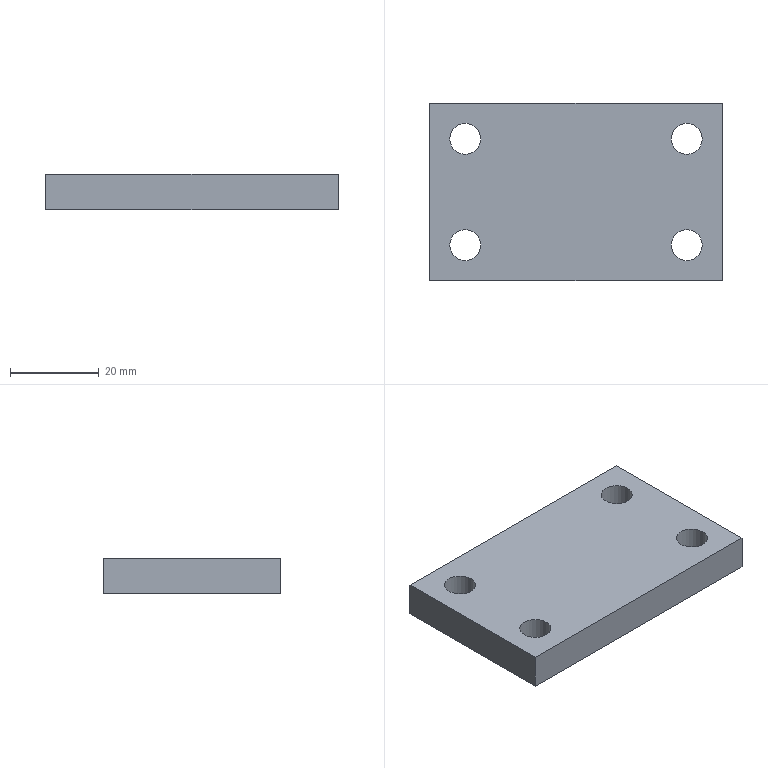Part | STEP file | Tube feed_id1018_x_t | 1 solid | 10 faces | box 66 x 40 x 8 mm | volume 19888 mm3 | plane 6 | cylinder 4 | commonest cylinder face diameters 7 x4
STEP:
#1=CARTESIAN_POINT('',(0.,0.,0.));
#2=DIRECTION('',(0.,0.,1.));
#3=DIRECTION('',(1.,0.,0.));
#4=AXIS2_PLACEMENT_3D('',#1,#2,#3);
#5=CARTESIAN_POINT('',(-297.,53.975,-133.5));
#6=VERTEX_POINT('',#5);
#7=CARTESIAN_POINT('',(-293.5,53.975,-133.5));
#8=DIRECTION('',(0.,0.,-1.));
#9=DIRECTION('',(-1.,0.,0.));
#10=AXIS2_PLACEMENT_3D('',#7,#8,#9);
#11=CIRCLE('',#10,3.5);
#12=CARTESIAN_POINT('',(-235.5,21.975,-133.5));
#13=DIRECTION('',(0.,0.,1.));
#14=DIRECTION('',(-1.,0.,0.));
#15=AXIS2_PLACEMENT_3D('',#12,#13,#14);
#16=PLANE('',#15);
#17=CARTESIAN_POINT('',(61.5,-32.));
#18=CARTESIAN_POINT('',(61.5,-38.062));
#19=CARTESIAN_POINT('',(56.25,-35.031));
#20=CARTESIAN_POINT('',(51.,-32.));
#21=CARTESIAN_POINT('',(56.25,-28.969));
#22=CARTESIAN_POINT('',(61.5,-25.938));
#23=CARTESIAN_POINT('',(61.5,-32.));
#24=(BOUNDED_CURVE()B_SPLINE_CURVE(2,(#17,#18,#19,#20,#21,#22,#23),.UNSPECIFIED.,.T.,.F.)B_SPLINE_CURVE_WITH_KNOTS((1,2,2,2,2,1),(-2.094,0.,2.094,4.189,6.283,8.378),.UNSPECIFIED.)CURVE()GEOMETRIC_REPRESENTATION_ITEM()RATIONAL_B_SPLINE_CURVE((1.,0.5,1.,0.5,1.,0.5,1.))REPRESENTATION_ITEM(''));
#25=(GEOMETRIC_REPRESENTATION_CONTEXT(2)PARAMETRIC_REPRESENTATION_CONTEXT()REPRESENTATION_CONTEXT('',''));
#26=DEFINITIONAL_REPRESENTATION('',(#24),#25);
#27=PCURVE('',#16,#26);
#28=CARTESIAN_POINT('',(-293.5,53.975,-133.5));
#29=DIRECTION('',(0.,0.,-1.));
#30=DIRECTION('',(-1.,0.,0.));
#31=AXIS2_PLACEMENT_3D('',#28,#29,#30);
#32=CYLINDRICAL_SURFACE('',#31,3.5);
#33=CARTESIAN_POINT('',(0.,0.));
#34=DIRECTION('',(1.,0.));
#35=VECTOR('',#34,1.);
#36=LINE('',#33,#35);
#37=(GEOMETRIC_REPRESENTATION_CONTEXT(2)PARAMETRIC_REPRESENTATION_CONTEXT()REPRESENTATION_CONTEXT('',''));
#38=DEFINITIONAL_REPRESENTATION('',(#36),#37);
#39=PCURVE('',#32,#38);
#40=SURFACE_CURVE('',#11,(#27,#39),.PCURVE_S1.);
#41=EDGE_CURVE('',#6,#6,#40,.T.);
#42=ORIENTED_EDGE('',*,*,#41,.T.);
#43=EDGE_LOOP('',(#42));
#44=FACE_BOUND('',#43,.T.);
#45=CARTESIAN_POINT('',(-297.,29.975,-133.5));
#46=VERTEX_POINT('',#45);
#47=CARTESIAN_POINT('',(-293.5,29.975,-133.5));
#48=DIRECTION('',(0.,0.,-1.));
#49=DIRECTION('',(-1.,0.,0.));
#50=AXIS2_PLACEMENT_3D('',#47,#48,#49);
#51=CIRCLE('',#50,3.5);
#52=CARTESIAN_POINT('',(61.5,-8.));
#53=CARTESIAN_POINT('',(61.5,-14.062));
#54=CARTESIAN_POINT('',(56.25,-11.031));
#55=CARTESIAN_POINT('',(51.,-8.));
#56=CARTESIAN_POINT('',(56.25,-4.969));
#57=CARTESIAN_POINT('',(61.5,-1.938));
#58=CARTESIAN_POINT('',(61.5,-8.));
#59=(BOUNDED_CURVE()B_SPLINE_CURVE(2,(#52,#53,#54,#55,#56,#57,#58),.UNSPECIFIED.,.T.,.F.)B_SPLINE_CURVE_WITH_KNOTS((1,2,2,2,2,1),(-2.094,0.,2.094,4.189,6.283,8.378),.UNSPECIFIED.)CURVE()GEOMETRIC_REPRESENTATION_ITEM()RATIONAL_B_SPLINE_CURVE((1.,0.5,1.,0.5,1.,0.5,1.))REPRESENTATION_ITEM(''));
#60=(GEOMETRIC_REPRESENTATION_CONTEXT(2)PARAMETRIC_REPRESENTATION_CONTEXT()REPRESENTATION_CONTEXT('',''));
#61=DEFINITIONAL_REPRESENTATION('',(#59),#60);
#62=PCURVE('',#16,#61);
#63=CARTESIAN_POINT('',(-293.5,29.975,-133.5));
#64=DIRECTION('',(0.,0.,-1.));
#65=DIRECTION('',(-1.,0.,0.));
#66=AXIS2_PLACEMENT_3D('',#63,#64,#65);
#67=CYLINDRICAL_SURFACE('',#66,3.5);
#68=CARTESIAN_POINT('',(0.,0.));
#69=DIRECTION('',(1.,0.));
#70=VECTOR('',#69,1.);
#71=LINE('',#68,#70);
#72=(GEOMETRIC_REPRESENTATION_CONTEXT(2)PARAMETRIC_REPRESENTATION_CONTEXT()REPRESENTATION_CONTEXT('',''));
#73=DEFINITIONAL_REPRESENTATION('',(#71),#72);
#74=PCURVE('',#67,#73);
#75=SURFACE_CURVE('',#51,(#62,#74),.PCURVE_S1.);
#76=EDGE_CURVE('',#46,#46,#75,.T.);
#77=ORIENTED_EDGE('',*,*,#76,.T.);
#78=EDGE_LOOP('',(#77));
#79=FACE_BOUND('',#78,.T.);
#80=CARTESIAN_POINT('',(-247.,29.975,-133.5));
#81=VERTEX_POINT('',#80);
#82=CARTESIAN_POINT('',(-243.5,29.975,-133.5));
#83=DIRECTION('',(0.,0.,-1.));
#84=DIRECTION('',(-1.,0.,0.));
#85=AXIS2_PLACEMENT_3D('',#82,#83,#84);
#86=CIRCLE('',#85,3.5);
#87=CARTESIAN_POINT('',(11.5,-8.));
#88=CARTESIAN_POINT('',(11.5,-14.062));
#89=CARTESIAN_POINT('',(6.25,-11.031));
#90=CARTESIAN_POINT('',(1.,-8.));
#91=CARTESIAN_POINT('',(6.25,-4.969));
#92=CARTESIAN_POINT('',(11.5,-1.938));
#93=CARTESIAN_POINT('',(11.5,-8.));
#94=(BOUNDED_CURVE()B_SPLINE_CURVE(2,(#87,#88,#89,#90,#91,#92,#93),.UNSPECIFIED.,.T.,.F.)B_SPLINE_CURVE_WITH_KNOTS((1,2,2,2,2,1),(-2.094,0.,2.094,4.189,6.283,8.378),.UNSPECIFIED.)CURVE()GEOMETRIC_REPRESENTATION_ITEM()RATIONAL_B_SPLINE_CURVE((1.,0.5,1.,0.5,1.,0.5,1.))REPRESENTATION_ITEM(''));
#95=(GEOMETRIC_REPRESENTATION_CONTEXT(2)PARAMETRIC_REPRESENTATION_CONTEXT()REPRESENTATION_CONTEXT('',''));
#96=DEFINITIONAL_REPRESENTATION('',(#94),#95);
#97=PCURVE('',#16,#96);
#98=CARTESIAN_POINT('',(-243.5,29.975,-133.5));
#99=DIRECTION('',(0.,0.,-1.));
#100=DIRECTION('',(-1.,0.,0.));
#101=AXIS2_PLACEMENT_3D('',#98,#99,#100);
#102=CYLINDRICAL_SURFACE('',#101,3.5);
#103=CARTESIAN_POINT('',(0.,0.));
#104=DIRECTION('',(1.,0.));
#105=VECTOR('',#104,1.);
#106=LINE('',#103,#105);
#107=(GEOMETRIC_REPRESENTATION_CONTEXT(2)PARAMETRIC_REPRESENTATION_CONTEXT()REPRESENTATION_CONTEXT('',''));
#108=DEFINITIONAL_REPRESENTATION('',(#106),#107);
#109=PCURVE('',#102,#108);
#110=SURFACE_CURVE('',#86,(#97,#109),.PCURVE_S1.);
#111=EDGE_CURVE('',#81,#81,#110,.T.);
#112=ORIENTED_EDGE('',*,*,#111,.T.);
#113=EDGE_LOOP('',(#112));
#114=FACE_BOUND('',#113,.T.);
#115=CARTESIAN_POINT('',(-247.,53.975,-133.5));
#116=VERTEX_POINT('',#115);
#117=CARTESIAN_POINT('',(-243.5,53.975,-133.5));
#118=DIRECTION('',(0.,0.,-1.));
#119=DIRECTION('',(-1.,0.,0.));
#120=AXIS2_PLACEMENT_3D('',#117,#118,#119);
#121=CIRCLE('',#120,3.5);
#122=CARTESIAN_POINT('',(11.5,-32.));
#123=CARTESIAN_POINT('',(11.5,-38.062));
#124=CARTESIAN_POINT('',(6.25,-35.031));
#125=CARTESIAN_POINT('',(1.,-32.));
#126=CARTESIAN_POINT('',(6.25,-28.969));
#127=CARTESIAN_POINT('',(11.5,-25.938));
#128=CARTESIAN_POINT('',(11.5,-32.));
#129=(BOUNDED_CURVE()B_SPLINE_CURVE(2,(#122,#123,#124,#125,#126,#127,#128),.UNSPECIFIED.,.T.,.F.)B_SPLINE_CURVE_WITH_KNOTS((1,2,2,2,2,1),(-2.094,0.,2.094,4.189,6.283,8.378),.UNSPECIFIED.)CURVE()GEOMETRIC_REPRESENTATION_ITEM()RATIONAL_B_SPLINE_CURVE((1.,0.5,1.,0.5,1.,0.5,1.))REPRESENTATION_ITEM(''));
#130=(GEOMETRIC_REPRESENTATION_CONTEXT(2)PARAMETRIC_REPRESENTATION_CONTEXT()REPRESENTATION_CONTEXT('',''));
#131=DEFINITIONAL_REPRESENTATION('',(#129),#130);
#132=PCURVE('',#16,#131);
#133=CARTESIAN_POINT('',(-243.5,53.975,-133.5));
#134=DIRECTION('',(0.,0.,-1.));
#135=DIRECTION('',(-1.,0.,0.));
#136=AXIS2_PLACEMENT_3D('',#133,#134,#135);
#137=CYLINDRICAL_SURFACE('',#136,3.5);
#138=CARTESIAN_POINT('',(0.,0.));
#139=DIRECTION('',(1.,0.));
#140=VECTOR('',#139,1.);
#141=LINE('',#138,#140);
#142=(GEOMETRIC_REPRESENTATION_CONTEXT(2)PARAMETRIC_REPRESENTATION_CONTEXT()REPRESENTATION_CONTEXT('',''));
#143=DEFINITIONAL_REPRESENTATION('',(#141),#142);
#144=PCURVE('',#137,#143);
#145=SURFACE_CURVE('',#121,(#132,#144),.PCURVE_S1.);
#146=EDGE_CURVE('',#116,#116,#145,.T.);
#147=ORIENTED_EDGE('',*,*,#146,.T.);
#148=EDGE_LOOP('',(#147));
#149=FACE_BOUND('',#148,.T.);
#150=CARTESIAN_POINT('',(-301.5,61.975,-133.5));
#151=VERTEX_POINT('',#150);
#152=CARTESIAN_POINT('',(-301.5,21.975,-133.5));
#153=VERTEX_POINT('',#152);
#154=CARTESIAN_POINT('',(-301.5,21.975,-133.5));
#155=DIRECTION('',(0.,-1.,0.));
#156=VECTOR('',#155,1.);
#157=LINE('',#154,#156);
#158=CARTESIAN_POINT('',(66.,0.));
#159=DIRECTION('',(0.,1.));
#160=VECTOR('',#159,1.);
#161=LINE('',#158,#160);
#162=(GEOMETRIC_REPRESENTATION_CONTEXT(2)PARAMETRIC_REPRESENTATION_CONTEXT()REPRESENTATION_CONTEXT('',''));
#163=DEFINITIONAL_REPRESENTATION('',(#161),#162);
#164=PCURVE('',#16,#163);
#165=CARTESIAN_POINT('',(-301.5,21.975,-133.5));
#166=DIRECTION('',(-1.,0.,0.));
#167=DIRECTION('',(0.,0.,-1.));
#168=AXIS2_PLACEMENT_3D('',#165,#166,#167);
#169=PLANE('',#168);
#170=CARTESIAN_POINT('',(0.,0.));
#171=DIRECTION('',(0.,1.));
#172=VECTOR('',#171,1.);
#173=LINE('',#170,#172);
#174=(GEOMETRIC_REPRESENTATION_CONTEXT(2)PARAMETRIC_REPRESENTATION_CONTEXT()REPRESENTATION_CONTEXT('',''));
#175=DEFINITIONAL_REPRESENTATION('',(#173),#174);
#176=PCURVE('',#169,#175);
#177=SURFACE_CURVE('',#157,(#164,#176),.PCURVE_S1.);
#178=EDGE_CURVE('',#151,#153,#177,.T.);
#179=ORIENTED_EDGE('',*,*,#178,.T.);
#180=CARTESIAN_POINT('',(-235.5,21.975,-133.5));
#181=VERTEX_POINT('',#180);
#182=CARTESIAN_POINT('',(-235.5,21.975,-133.5));
#183=DIRECTION('',(1.,0.,0.));
#184=VECTOR('',#183,1.);
#185=LINE('',#182,#184);
#186=CARTESIAN_POINT('',(0.,0.));
#187=DIRECTION('',(-1.,0.));
#188=VECTOR('',#187,1.);
#189=LINE('',#186,#188);
#190=(GEOMETRIC_REPRESENTATION_CONTEXT(2)PARAMETRIC_REPRESENTATION_CONTEXT()REPRESENTATION_CONTEXT('',''));
#191=DEFINITIONAL_REPRESENTATION('',(#189),#190);
#192=PCURVE('',#16,#191);
#193=CARTESIAN_POINT('',(-235.5,21.975,-133.5));
#194=DIRECTION('',(0.,-1.,0.));
#195=DIRECTION('',(1.,0.,0.));
#196=AXIS2_PLACEMENT_3D('',#193,#194,#195);
#197=PLANE('',#196);
#198=CARTESIAN_POINT('',(0.,0.));
#199=DIRECTION('',(1.,0.));
#200=VECTOR('',#199,1.);
#201=LINE('',#198,#200);
#202=(GEOMETRIC_REPRESENTATION_CONTEXT(2)PARAMETRIC_REPRESENTATION_CONTEXT()REPRESENTATION_CONTEXT('',''));
#203=DEFINITIONAL_REPRESENTATION('',(#201),#202);
#204=PCURVE('',#197,#203);
#205=SURFACE_CURVE('',#185,(#192,#204),.PCURVE_S1.);
#206=EDGE_CURVE('',#153,#181,#205,.T.);
#207=ORIENTED_EDGE('',*,*,#206,.T.);
#208=CARTESIAN_POINT('',(-235.5,61.975,-133.5));
#209=VERTEX_POINT('',#208);
#210=CARTESIAN_POINT('',(-235.5,21.975,-133.5));
#211=DIRECTION('',(0.,-1.,0.));
#212=VECTOR('',#211,1.);
#213=LINE('',#210,#212);
#214=CARTESIAN_POINT('',(0.,0.));
#215=DIRECTION('',(0.,1.));
#216=VECTOR('',#215,1.);
#217=LINE('',#214,#216);
#218=(GEOMETRIC_REPRESENTATION_CONTEXT(2)PARAMETRIC_REPRESENTATION_CONTEXT()REPRESENTATION_CONTEXT('',''));
#219=DEFINITIONAL_REPRESENTATION('',(#217),#218);
#220=PCURVE('',#16,#219);
#221=CARTESIAN_POINT('',(-235.5,21.975,-133.5));
#222=DIRECTION('',(-1.,0.,0.));
#223=DIRECTION('',(0.,0.,-1.));
#224=AXIS2_PLACEMENT_3D('',#221,#222,#223);
#225=PLANE('',#224);
#226=CARTESIAN_POINT('',(0.,0.));
#227=DIRECTION('',(0.,1.));
#228=VECTOR('',#227,1.);
#229=LINE('',#226,#228);
#230=(GEOMETRIC_REPRESENTATION_CONTEXT(2)PARAMETRIC_REPRESENTATION_CONTEXT()REPRESENTATION_CONTEXT('',''));
#231=DEFINITIONAL_REPRESENTATION('',(#229),#230);
#232=PCURVE('',#225,#231);
#233=SURFACE_CURVE('',#213,(#220,#232),.PCURVE_S1.);
#234=EDGE_CURVE('',#209,#181,#233,.T.);
#235=ORIENTED_EDGE('',*,*,#234,.F.);
#236=CARTESIAN_POINT('',(-235.5,61.975,-133.5));
#237=DIRECTION('',(1.,0.,0.));
#238=VECTOR('',#237,1.);
#239=LINE('',#236,#238);
#240=CARTESIAN_POINT('',(0.,-40.));
#241=DIRECTION('',(-1.,0.));
#242=VECTOR('',#241,1.);
#243=LINE('',#240,#242);
#244=(GEOMETRIC_REPRESENTATION_CONTEXT(2)PARAMETRIC_REPRESENTATION_CONTEXT()REPRESENTATION_CONTEXT('',''));
#245=DEFINITIONAL_REPRESENTATION('',(#243),#244);
#246=PCURVE('',#16,#245);
#247=CARTESIAN_POINT('',(-235.5,61.975,-133.5));
#248=DIRECTION('',(0.,-1.,0.));
#249=DIRECTION('',(1.,0.,0.));
#250=AXIS2_PLACEMENT_3D('',#247,#248,#249);
#251=PLANE('',#250);
#252=CARTESIAN_POINT('',(0.,0.));
#253=DIRECTION('',(1.,0.));
#254=VECTOR('',#253,1.);
#255=LINE('',#252,#254);
#256=(GEOMETRIC_REPRESENTATION_CONTEXT(2)PARAMETRIC_REPRESENTATION_CONTEXT()REPRESENTATION_CONTEXT('',''));
#257=DEFINITIONAL_REPRESENTATION('',(#255),#256);
#258=PCURVE('',#251,#257);
#259=SURFACE_CURVE('',#239,(#246,#258),.PCURVE_S1.);
#260=EDGE_CURVE('',#151,#209,#259,.T.);
#261=ORIENTED_EDGE('',*,*,#260,.F.);
#262=EDGE_LOOP('',(#179,#207,#235,#261));
#263=FACE_BOUND('',#262,.T.);
#264=ADVANCED_FACE('',(#44,#79,#114,#149,#263),#16,.T.);
#265=ORIENTED_EDGE('',*,*,#234,.T.);
#266=CARTESIAN_POINT('',(-235.5,21.975,-141.5));
#267=VERTEX_POINT('',#266);
#268=CARTESIAN_POINT('',(-235.5,21.975,-133.5));
#269=DIRECTION('',(0.,0.,-1.));
#270=VECTOR('',#269,1.);
#271=LINE('',#268,#270);
#272=CARTESIAN_POINT('',(0.,0.));
#273=DIRECTION('',(1.,0.));
#274=VECTOR('',#273,1.);
#275=LINE('',#272,#274);
#276=(GEOMETRIC_REPRESENTATION_CONTEXT(2)PARAMETRIC_REPRESENTATION_CONTEXT()REPRESENTATION_CONTEXT('',''));
#277=DEFINITIONAL_REPRESENTATION('',(#275),#276);
#278=PCURVE('',#225,#277);
#279=CARTESIAN_POINT('',(0.,0.));
#280=DIRECTION('',(0.,-1.));
#281=VECTOR('',#280,1.);
#282=LINE('',#279,#281);
#283=(GEOMETRIC_REPRESENTATION_CONTEXT(2)PARAMETRIC_REPRESENTATION_CONTEXT()REPRESENTATION_CONTEXT('',''));
#284=DEFINITIONAL_REPRESENTATION('',(#282),#283);
#285=PCURVE('',#197,#284);
#286=SURFACE_CURVE('',#271,(#278,#285),.PCURVE_S1.);
#287=EDGE_CURVE('',#181,#267,#286,.T.);
#288=ORIENTED_EDGE('',*,*,#287,.T.);
#289=CARTESIAN_POINT('',(-235.5,61.975,-141.5));
#290=VERTEX_POINT('',#289);
#291=CARTESIAN_POINT('',(-235.5,21.975,-141.5));
#292=DIRECTION('',(0.,-1.,0.));
#293=VECTOR('',#292,1.);
#294=LINE('',#291,#293);
#295=CARTESIAN_POINT('',(8.,0.));
#296=DIRECTION('',(0.,1.));
#297=VECTOR('',#296,1.);
#298=LINE('',#295,#297);
#299=(GEOMETRIC_REPRESENTATION_CONTEXT(2)PARAMETRIC_REPRESENTATION_CONTEXT()REPRESENTATION_CONTEXT('',''));
#300=DEFINITIONAL_REPRESENTATION('',(#298),#299);
#301=PCURVE('',#225,#300);
#302=CARTESIAN_POINT('',(-235.5,21.975,-141.5));
#303=DIRECTION('',(0.,0.,1.));
#304=DIRECTION('',(-1.,0.,0.));
#305=AXIS2_PLACEMENT_3D('',#302,#303,#304);
#306=PLANE('',#305);
#307=CARTESIAN_POINT('',(0.,0.));
#308=DIRECTION('',(0.,1.));
#309=VECTOR('',#308,1.);
#310=LINE('',#307,#309);
#311=(GEOMETRIC_REPRESENTATION_CONTEXT(2)PARAMETRIC_REPRESENTATION_CONTEXT()REPRESENTATION_CONTEXT('',''));
#312=DEFINITIONAL_REPRESENTATION('',(#310),#311);
#313=PCURVE('',#306,#312);
#314=SURFACE_CURVE('',#294,(#301,#313),.PCURVE_S1.);
#315=EDGE_CURVE('',#290,#267,#314,.T.);
#316=ORIENTED_EDGE('',*,*,#315,.F.);
#317=CARTESIAN_POINT('',(-235.5,61.975,-133.5));
#318=DIRECTION('',(0.,0.,-1.));
#319=VECTOR('',#318,1.);
#320=LINE('',#317,#319);
#321=CARTESIAN_POINT('',(0.,-40.));
#322=DIRECTION('',(1.,0.));
#323=VECTOR('',#322,1.);
#324=LINE('',#321,#323);
#325=(GEOMETRIC_REPRESENTATION_CONTEXT(2)PARAMETRIC_REPRESENTATION_CONTEXT()REPRESENTATION_CONTEXT('',''));
#326=DEFINITIONAL_REPRESENTATION('',(#324),#325);
#327=PCURVE('',#225,#326);
#328=CARTESIAN_POINT('',(0.,0.));
#329=DIRECTION('',(0.,-1.));
#330=VECTOR('',#329,1.);
#331=LINE('',#328,#330);
#332=(GEOMETRIC_REPRESENTATION_CONTEXT(2)PARAMETRIC_REPRESENTATION_CONTEXT()REPRESENTATION_CONTEXT('',''));
#333=DEFINITIONAL_REPRESENTATION('',(#331),#332);
#334=PCURVE('',#251,#333);
#335=SURFACE_CURVE('',#320,(#327,#334),.PCURVE_S1.);
#336=EDGE_CURVE('',#209,#290,#335,.T.);
#337=ORIENTED_EDGE('',*,*,#336,.F.);
#338=EDGE_LOOP('',(#265,#288,#316,#337));
#339=FACE_BOUND('',#338,.T.);
#340=ADVANCED_FACE('',(#339),#225,.F.);
#341=CARTESIAN_POINT('',(-290.,53.975,-141.5));
#342=VERTEX_POINT('',#341);
#343=CARTESIAN_POINT('',(-297.,53.975,-141.5));
#344=VERTEX_POINT('',#343);
#345=CARTESIAN_POINT('',(-293.5,53.975,-141.5));
#346=DIRECTION('',(0.,0.,1.));
#347=DIRECTION('',(1.,0.,0.));
#348=AXIS2_PLACEMENT_3D('',#345,#346,#347);
#349=CIRCLE('',#348,3.5);
#350=CARTESIAN_POINT('',(58.,-32.));
#351=DIRECTION('',(-1.,0.));
#352=AXIS2_PLACEMENT_2D('',#350,#351);
#353=CIRCLE('',#352,3.5);
#354=(GEOMETRIC_REPRESENTATION_CONTEXT(2)PARAMETRIC_REPRESENTATION_CONTEXT()REPRESENTATION_CONTEXT('',''));
#355=DEFINITIONAL_REPRESENTATION('',(#353),#354);
#356=PCURVE('',#306,#355);
#357=CARTESIAN_POINT('',(3.142,8.));
#358=DIRECTION('',(-1.,0.));
#359=VECTOR('',#358,1.);
#360=LINE('',#357,#359);
#361=(GEOMETRIC_REPRESENTATION_CONTEXT(2)PARAMETRIC_REPRESENTATION_CONTEXT()REPRESENTATION_CONTEXT('',''));
#362=DEFINITIONAL_REPRESENTATION('',(#360),#361);
#363=PCURVE('',#32,#362);
#364=SURFACE_CURVE('',#349,(#356,#363),.PCURVE_S1.);
#365=EDGE_CURVE('',#342,#344,#364,.T.);
#366=ORIENTED_EDGE('',*,*,#365,.T.);
#367=CARTESIAN_POINT('',(-293.5,53.975,-141.5));
#368=DIRECTION('',(0.,0.,1.));
#369=DIRECTION('',(1.,0.,0.));
#370=AXIS2_PLACEMENT_3D('',#367,#368,#369);
#371=CIRCLE('',#370,3.5);
#372=CARTESIAN_POINT('',(58.,-32.));
#373=DIRECTION('',(-1.,0.));
#374=AXIS2_PLACEMENT_2D('',#372,#373);
#375=CIRCLE('',#374,3.5);
#376=(GEOMETRIC_REPRESENTATION_CONTEXT(2)PARAMETRIC_REPRESENTATION_CONTEXT()REPRESENTATION_CONTEXT('',''));
#377=DEFINITIONAL_REPRESENTATION('',(#375),#376);
#378=PCURVE('',#306,#377);
#379=CARTESIAN_POINT('',(9.425,8.));
#380=DIRECTION('',(-1.,0.));
#381=VECTOR('',#380,1.);
#382=LINE('',#379,#381);
#383=(GEOMETRIC_REPRESENTATION_CONTEXT(2)PARAMETRIC_REPRESENTATION_CONTEXT()REPRESENTATION_CONTEXT('',''));
#384=DEFINITIONAL_REPRESENTATION('',(#382),#383);
#385=PCURVE('',#32,#384);
#386=SURFACE_CURVE('',#371,(#378,#385),.PCURVE_S1.);
#387=EDGE_CURVE('',#344,#342,#386,.T.);
#388=ORIENTED_EDGE('',*,*,#387,.T.);
#389=EDGE_LOOP('',(#366,#388));
#390=FACE_BOUND('',#389,.T.);
#391=CARTESIAN_POINT('',(-290.,29.975,-141.5));
#392=VERTEX_POINT('',#391);
#393=CARTESIAN_POINT('',(-297.,29.975,-141.5));
#394=VERTEX_POINT('',#393);
#395=CARTESIAN_POINT('',(-293.5,29.975,-141.5));
#396=DIRECTION('',(0.,0.,1.));
#397=DIRECTION('',(1.,0.,0.));
#398=AXIS2_PLACEMENT_3D('',#395,#396,#397);
#399=CIRCLE('',#398,3.5);
#400=CARTESIAN_POINT('',(58.,-8.));
#401=DIRECTION('',(-1.,0.));
#402=AXIS2_PLACEMENT_2D('',#400,#401);
#403=CIRCLE('',#402,3.5);
#404=(GEOMETRIC_REPRESENTATION_CONTEXT(2)PARAMETRIC_REPRESENTATION_CONTEXT()REPRESENTATION_CONTEXT('',''));
#405=DEFINITIONAL_REPRESENTATION('',(#403),#404);
#406=PCURVE('',#306,#405);
#407=CARTESIAN_POINT('',(3.142,8.));
#408=DIRECTION('',(-1.,0.));
#409=VECTOR('',#408,1.);
#410=LINE('',#407,#409);
#411=(GEOMETRIC_REPRESENTATION_CONTEXT(2)PARAMETRIC_REPRESENTATION_CONTEXT()REPRESENTATION_CONTEXT('',''));
#412=DEFINITIONAL_REPRESENTATION('',(#410),#411);
#413=PCURVE('',#67,#412);
#414=SURFACE_CURVE('',#399,(#406,#413),.PCURVE_S1.);
#415=EDGE_CURVE('',#392,#394,#414,.T.);
#416=ORIENTED_EDGE('',*,*,#415,.T.);
#417=CARTESIAN_POINT('',(-293.5,29.975,-141.5));
#418=DIRECTION('',(0.,0.,1.));
#419=DIRECTION('',(1.,0.,0.));
#420=AXIS2_PLACEMENT_3D('',#417,#418,#419);
#421=CIRCLE('',#420,3.5);
#422=CARTESIAN_POINT('',(58.,-8.));
#423=DIRECTION('',(-1.,0.));
#424=AXIS2_PLACEMENT_2D('',#422,#423);
#425=CIRCLE('',#424,3.5);
#426=(GEOMETRIC_REPRESENTATION_CONTEXT(2)PARAMETRIC_REPRESENTATION_CONTEXT()REPRESENTATION_CONTEXT('',''));
#427=DEFINITIONAL_REPRESENTATION('',(#425),#426);
#428=PCURVE('',#306,#427);
#429=CARTESIAN_POINT('',(9.425,8.));
#430=DIRECTION('',(-1.,0.));
#431=VECTOR('',#430,1.);
#432=LINE('',#429,#431);
#433=(GEOMETRIC_REPRESENTATION_CONTEXT(2)PARAMETRIC_REPRESENTATION_CONTEXT()REPRESENTATION_CONTEXT('',''));
#434=DEFINITIONAL_REPRESENTATION('',(#432),#433);
#435=PCURVE('',#67,#434);
#436=SURFACE_CURVE('',#421,(#428,#435),.PCURVE_S1.);
#437=EDGE_CURVE('',#394,#392,#436,.T.);
#438=ORIENTED_EDGE('',*,*,#437,.T.);
#439=EDGE_LOOP('',(#416,#438));
#440=FACE_BOUND('',#439,.T.);
#441=CARTESIAN_POINT('',(-240.,29.975,-141.5));
#442=VERTEX_POINT('',#441);
#443=CARTESIAN_POINT('',(-247.,29.975,-141.5));
#444=VERTEX_POINT('',#443);
#445=CARTESIAN_POINT('',(-243.5,29.975,-141.5));
#446=DIRECTION('',(0.,0.,1.));
#447=DIRECTION('',(1.,0.,0.));
#448=AXIS2_PLACEMENT_3D('',#445,#446,#447);
#449=CIRCLE('',#448,3.5);
#450=CARTESIAN_POINT('',(8.,-8.));
#451=DIRECTION('',(-1.,0.));
#452=AXIS2_PLACEMENT_2D('',#450,#451);
#453=CIRCLE('',#452,3.5);
#454=(GEOMETRIC_REPRESENTATION_CONTEXT(2)PARAMETRIC_REPRESENTATION_CONTEXT()REPRESENTATION_CONTEXT('',''));
#455=DEFINITIONAL_REPRESENTATION('',(#453),#454);
#456=PCURVE('',#306,#455);
#457=CARTESIAN_POINT('',(3.142,8.));
#458=DIRECTION('',(-1.,0.));
#459=VECTOR('',#458,1.);
#460=LINE('',#457,#459);
#461=(GEOMETRIC_REPRESENTATION_CONTEXT(2)PARAMETRIC_REPRESENTATION_CONTEXT()REPRESENTATION_CONTEXT('',''));
#462=DEFINITIONAL_REPRESENTATION('',(#460),#461);
#463=PCURVE('',#102,#462);
#464=SURFACE_CURVE('',#449,(#456,#463),.PCURVE_S1.);
#465=EDGE_CURVE('',#442,#444,#464,.T.);
#466=ORIENTED_EDGE('',*,*,#465,.T.);
#467=CARTESIAN_POINT('',(-243.5,29.975,-141.5));
#468=DIRECTION('',(0.,0.,1.));
#469=DIRECTION('',(1.,0.,0.));
#470=AXIS2_PLACEMENT_3D('',#467,#468,#469);
#471=CIRCLE('',#470,3.5);
#472=CARTESIAN_POINT('',(8.,-8.));
#473=DIRECTION('',(-1.,0.));
#474=AXIS2_PLACEMENT_2D('',#472,#473);
#475=CIRCLE('',#474,3.5);
#476=(GEOMETRIC_REPRESENTATION_CONTEXT(2)PARAMETRIC_REPRESENTATION_CONTEXT()REPRESENTATION_CONTEXT('',''));
#477=DEFINITIONAL_REPRESENTATION('',(#475),#476);
#478=PCURVE('',#306,#477);
#479=CARTESIAN_POINT('',(9.425,8.));
#480=DIRECTION('',(-1.,0.));
#481=VECTOR('',#480,1.);
#482=LINE('',#479,#481);
#483=(GEOMETRIC_REPRESENTATION_CONTEXT(2)PARAMETRIC_REPRESENTATION_CONTEXT()REPRESENTATION_CONTEXT('',''));
#484=DEFINITIONAL_REPRESENTATION('',(#482),#483);
#485=PCURVE('',#102,#484);
#486=SURFACE_CURVE('',#471,(#478,#485),.PCURVE_S1.);
#487=EDGE_CURVE('',#444,#442,#486,.T.);
#488=ORIENTED_EDGE('',*,*,#487,.T.);
#489=EDGE_LOOP('',(#466,#488));
#490=FACE_BOUND('',#489,.T.);
#491=CARTESIAN_POINT('',(-240.,53.975,-141.5));
#492=VERTEX_POINT('',#491);
#493=CARTESIAN_POINT('',(-247.,53.975,-141.5));
#494=VERTEX_POINT('',#493);
#495=CARTESIAN_POINT('',(-243.5,53.975,-141.5));
#496=DIRECTION('',(0.,0.,1.));
#497=DIRECTION('',(1.,0.,0.));
#498=AXIS2_PLACEMENT_3D('',#495,#496,#497);
#499=CIRCLE('',#498,3.5);
#500=CARTESIAN_POINT('',(8.,-32.));
#501=DIRECTION('',(-1.,0.));
#502=AXIS2_PLACEMENT_2D('',#500,#501);
#503=CIRCLE('',#502,3.5);
#504=(GEOMETRIC_REPRESENTATION_CONTEXT(2)PARAMETRIC_REPRESENTATION_CONTEXT()REPRESENTATION_CONTEXT('',''));
#505=DEFINITIONAL_REPRESENTATION('',(#503),#504);
#506=PCURVE('',#306,#505);
#507=CARTESIAN_POINT('',(3.142,8.));
#508=DIRECTION('',(-1.,0.));
#509=VECTOR('',#508,1.);
#510=LINE('',#507,#509);
#511=(GEOMETRIC_REPRESENTATION_CONTEXT(2)PARAMETRIC_REPRESENTATION_CONTEXT()REPRESENTATION_CONTEXT('',''));
#512=DEFINITIONAL_REPRESENTATION('',(#510),#511);
#513=PCURVE('',#137,#512);
#514=SURFACE_CURVE('',#499,(#506,#513),.PCURVE_S1.);
#515=EDGE_CURVE('',#492,#494,#514,.T.);
#516=ORIENTED_EDGE('',*,*,#515,.T.);
#517=CARTESIAN_POINT('',(-243.5,53.975,-141.5));
#518=DIRECTION('',(0.,0.,1.));
#519=DIRECTION('',(1.,0.,0.));
#520=AXIS2_PLACEMENT_3D('',#517,#518,#519);
#521=CIRCLE('',#520,3.5);
#522=CARTESIAN_POINT('',(8.,-32.));
#523=DIRECTION('',(-1.,0.));
#524=AXIS2_PLACEMENT_2D('',#522,#523);
#525=CIRCLE('',#524,3.5);
#526=(GEOMETRIC_REPRESENTATION_CONTEXT(2)PARAMETRIC_REPRESENTATION_CONTEXT()REPRESENTATION_CONTEXT('',''));
#527=DEFINITIONAL_REPRESENTATION('',(#525),#526);
#528=PCURVE('',#306,#527);
#529=CARTESIAN_POINT('',(9.425,8.));
#530=DIRECTION('',(-1.,0.));
#531=VECTOR('',#530,1.);
#532=LINE('',#529,#531);
#533=(GEOMETRIC_REPRESENTATION_CONTEXT(2)PARAMETRIC_REPRESENTATION_CONTEXT()REPRESENTATION_CONTEXT('',''));
#534=DEFINITIONAL_REPRESENTATION('',(#532),#533);
#535=PCURVE('',#137,#534);
#536=SURFACE_CURVE('',#521,(#528,#535),.PCURVE_S1.);
#537=EDGE_CURVE('',#494,#492,#536,.T.);
#538=ORIENTED_EDGE('',*,*,#537,.T.);
#539=EDGE_LOOP('',(#516,#538));
#540=FACE_BOUND('',#539,.T.);
#541=ORIENTED_EDGE('',*,*,#315,.T.);
#542=CARTESIAN_POINT('',(-301.5,21.975,-141.5));
#543=VERTEX_POINT('',#542);
#544=CARTESIAN_POINT('',(-235.5,21.975,-141.5));
#545=DIRECTION('',(-1.,0.,0.));
#546=VECTOR('',#545,1.);
#547=LINE('',#544,#546);
#548=CARTESIAN_POINT('',(0.,0.));
#549=DIRECTION('',(1.,0.));
#550=VECTOR('',#549,1.);
#551=LINE('',#548,#550);
#552=(GEOMETRIC_REPRESENTATION_CONTEXT(2)PARAMETRIC_REPRESENTATION_CONTEXT()REPRESENTATION_CONTEXT('',''));
#553=DEFINITIONAL_REPRESENTATION('',(#551),#552);
#554=PCURVE('',#306,#553);
#555=CARTESIAN_POINT('',(0.,-8.));
#556=DIRECTION('',(-1.,0.));
#557=VECTOR('',#556,1.);
#558=LINE('',#555,#557);
#559=(GEOMETRIC_REPRESENTATION_CONTEXT(2)PARAMETRIC_REPRESENTATION_CONTEXT()REPRESENTATION_CONTEXT('',''));
#560=DEFINITIONAL_REPRESENTATION('',(#558),#559);
#561=PCURVE('',#197,#560);
#562=SURFACE_CURVE('',#547,(#554,#561),.PCURVE_S1.);
#563=EDGE_CURVE('',#267,#543,#562,.T.);
#564=ORIENTED_EDGE('',*,*,#563,.T.);
#565=CARTESIAN_POINT('',(-301.5,61.975,-141.5));
#566=VERTEX_POINT('',#565);
#567=CARTESIAN_POINT('',(-301.5,21.975,-141.5));
#568=DIRECTION('',(0.,-1.,0.));
#569=VECTOR('',#568,1.);
#570=LINE('',#567,#569);
#571=CARTESIAN_POINT('',(66.,0.));
#572=DIRECTION('',(0.,1.));
#573=VECTOR('',#572,1.);
#574=LINE('',#571,#573);
#575=(GEOMETRIC_REPRESENTATION_CONTEXT(2)PARAMETRIC_REPRESENTATION_CONTEXT()REPRESENTATION_CONTEXT('',''));
#576=DEFINITIONAL_REPRESENTATION('',(#574),#575);
#577=PCURVE('',#306,#576);
#578=CARTESIAN_POINT('',(8.,0.));
#579=DIRECTION('',(0.,1.));
#580=VECTOR('',#579,1.);
#581=LINE('',#578,#580);
#582=(GEOMETRIC_REPRESENTATION_CONTEXT(2)PARAMETRIC_REPRESENTATION_CONTEXT()REPRESENTATION_CONTEXT('',''));
#583=DEFINITIONAL_REPRESENTATION('',(#581),#582);
#584=PCURVE('',#169,#583);
#585=SURFACE_CURVE('',#570,(#577,#584),.PCURVE_S1.);
#586=EDGE_CURVE('',#566,#543,#585,.T.);
#587=ORIENTED_EDGE('',*,*,#586,.F.);
#588=CARTESIAN_POINT('',(-235.5,61.975,-141.5));
#589=DIRECTION('',(-1.,0.,0.));
#590=VECTOR('',#589,1.);
#591=LINE('',#588,#590);
#592=CARTESIAN_POINT('',(0.,-40.));
#593=DIRECTION('',(1.,0.));
#594=VECTOR('',#593,1.);
#595=LINE('',#592,#594);
#596=(GEOMETRIC_REPRESENTATION_CONTEXT(2)PARAMETRIC_REPRESENTATION_CONTEXT()REPRESENTATION_CONTEXT('',''));
#597=DEFINITIONAL_REPRESENTATION('',(#595),#596);
#598=PCURVE('',#306,#597);
#599=CARTESIAN_POINT('',(0.,-8.));
#600=DIRECTION('',(-1.,0.));
#601=VECTOR('',#600,1.);
#602=LINE('',#599,#601);
#603=(GEOMETRIC_REPRESENTATION_CONTEXT(2)PARAMETRIC_REPRESENTATION_CONTEXT()REPRESENTATION_CONTEXT('',''));
#604=DEFINITIONAL_REPRESENTATION('',(#602),#603);
#605=PCURVE('',#251,#604);
#606=SURFACE_CURVE('',#591,(#598,#605),.PCURVE_S1.);
#607=EDGE_CURVE('',#290,#566,#606,.T.);
#608=ORIENTED_EDGE('',*,*,#607,.F.);
#609=EDGE_LOOP('',(#541,#564,#587,#608));
#610=FACE_BOUND('',#609,.T.);
#611=ADVANCED_FACE('',(#390,#440,#490,#540,#610),#306,.F.);
#612=CARTESIAN_POINT('',(-301.5,61.975,-133.5));
#613=DIRECTION('',(0.,0.,1.));
#614=VECTOR('',#613,1.);
#615=LINE('',#612,#614);
#616=CARTESIAN_POINT('',(0.,-40.));
#617=DIRECTION('',(-1.,0.));
#618=VECTOR('',#617,1.);
#619=LINE('',#616,#618);
#620=(GEOMETRIC_REPRESENTATION_CONTEXT(2)PARAMETRIC_REPRESENTATION_CONTEXT()REPRESENTATION_CONTEXT('',''));
#621=DEFINITIONAL_REPRESENTATION('',(#619),#620);
#622=PCURVE('',#169,#621);
#623=CARTESIAN_POINT('',(-66.,0.));
#624=DIRECTION('',(0.,1.));
#625=VECTOR('',#624,1.);
#626=LINE('',#623,#625);
#627=(GEOMETRIC_REPRESENTATION_CONTEXT(2)PARAMETRIC_REPRESENTATION_CONTEXT()REPRESENTATION_CONTEXT('',''));
#628=DEFINITIONAL_REPRESENTATION('',(#626),#627);
#629=PCURVE('',#251,#628);
#630=SURFACE_CURVE('',#615,(#622,#629),.PCURVE_S1.);
#631=EDGE_CURVE('',#566,#151,#630,.T.);
#632=ORIENTED_EDGE('',*,*,#631,.F.);
#633=ORIENTED_EDGE('',*,*,#586,.T.);
#634=CARTESIAN_POINT('',(-301.5,21.975,-133.5));
#635=DIRECTION('',(0.,0.,1.));
#636=VECTOR('',#635,1.);
#637=LINE('',#634,#636);
#638=CARTESIAN_POINT('',(0.,0.));
#639=DIRECTION('',(-1.,0.));
#640=VECTOR('',#639,1.);
#641=LINE('',#638,#640);
#642=(GEOMETRIC_REPRESENTATION_CONTEXT(2)PARAMETRIC_REPRESENTATION_CONTEXT()REPRESENTATION_CONTEXT('',''));
#643=DEFINITIONAL_REPRESENTATION('',(#641),#642);
#644=PCURVE('',#169,#643);
#645=CARTESIAN_POINT('',(-66.,0.));
#646=DIRECTION('',(0.,1.));
#647=VECTOR('',#646,1.);
#648=LINE('',#645,#647);
#649=(GEOMETRIC_REPRESENTATION_CONTEXT(2)PARAMETRIC_REPRESENTATION_CONTEXT()REPRESENTATION_CONTEXT('',''));
#650=DEFINITIONAL_REPRESENTATION('',(#648),#649);
#651=PCURVE('',#197,#650);
#652=SURFACE_CURVE('',#637,(#644,#651),.PCURVE_S1.);
#653=EDGE_CURVE('',#543,#153,#652,.T.);
#654=ORIENTED_EDGE('',*,*,#653,.T.);
#655=ORIENTED_EDGE('',*,*,#178,.F.);
#656=EDGE_LOOP('',(#632,#633,#654,#655));
#657=FACE_BOUND('',#656,.T.);
#658=ADVANCED_FACE('',(#657),#169,.T.);
#659=ORIENTED_EDGE('',*,*,#563,.F.);
#660=ORIENTED_EDGE('',*,*,#287,.F.);
#661=ORIENTED_EDGE('',*,*,#206,.F.);
#662=ORIENTED_EDGE('',*,*,#653,.F.);
#663=EDGE_LOOP('',(#659,#660,#661,#662));
#664=FACE_BOUND('',#663,.T.);
#665=ADVANCED_FACE('',(#664),#197,.T.);
#666=ORIENTED_EDGE('',*,*,#607,.T.);
#667=ORIENTED_EDGE('',*,*,#631,.T.);
#668=ORIENTED_EDGE('',*,*,#260,.T.);
#669=ORIENTED_EDGE('',*,*,#336,.T.);
#670=EDGE_LOOP('',(#666,#667,#668,#669));
#671=FACE_BOUND('',#670,.T.);
#672=ADVANCED_FACE('',(#671),#251,.F.);
#673=ORIENTED_EDGE('',*,*,#146,.T.);
#674=CARTESIAN_POINT('',(-247.,53.975,-133.5));
#675=CARTESIAN_POINT('',(-247.,53.975,-141.5));
#676=B_SPLINE_CURVE_WITH_KNOTS('',1,(#674,#675),.UNSPECIFIED.,.F.,.F.,(2,2),(0.,8.),.PIECEWISE_BEZIER_KNOTS.);
#677=CARTESIAN_POINT('',(6.283,0.));
#678=DIRECTION('',(0.,1.));
#679=VECTOR('',#678,1.);
#680=LINE('',#677,#679);
#681=(GEOMETRIC_REPRESENTATION_CONTEXT(2)PARAMETRIC_REPRESENTATION_CONTEXT()REPRESENTATION_CONTEXT('',''));
#682=DEFINITIONAL_REPRESENTATION('',(#680),#681);
#683=PCURVE('',#137,#682);
#684=CARTESIAN_POINT('',(0.,0.));
#685=DIRECTION('',(0.,1.));
#686=VECTOR('',#685,1.);
#687=LINE('',#684,#686);
#688=(GEOMETRIC_REPRESENTATION_CONTEXT(2)PARAMETRIC_REPRESENTATION_CONTEXT()REPRESENTATION_CONTEXT('',''));
#689=DEFINITIONAL_REPRESENTATION('',(#687),#688);
#690=PCURVE('',#137,#689);
#691=SEAM_CURVE('',#676,(#683,#690),.PCURVE_S1.);
#692=EDGE_CURVE('',#116,#494,#691,.T.);
#693=ORIENTED_EDGE('',*,*,#692,.T.);
#694=ORIENTED_EDGE('',*,*,#537,.T.);
#695=ORIENTED_EDGE('',*,*,#515,.T.);
#696=ORIENTED_EDGE('',*,*,#692,.F.);
#697=EDGE_LOOP('',(#673,#693,#694,#695,#696));
#698=FACE_BOUND('',#697,.F.);
#699=ADVANCED_FACE('',(#698),#137,.F.);
#700=ORIENTED_EDGE('',*,*,#111,.T.);
#701=CARTESIAN_POINT('',(-247.,29.975,-133.5));
#702=CARTESIAN_POINT('',(-247.,29.975,-141.5));
#703=B_SPLINE_CURVE_WITH_KNOTS('',1,(#701,#702),.UNSPECIFIED.,.F.,.F.,(2,2),(0.,8.),.PIECEWISE_BEZIER_KNOTS.);
#704=CARTESIAN_POINT('',(6.283,0.));
#705=DIRECTION('',(0.,1.));
#706=VECTOR('',#705,1.);
#707=LINE('',#704,#706);
#708=(GEOMETRIC_REPRESENTATION_CONTEXT(2)PARAMETRIC_REPRESENTATION_CONTEXT()REPRESENTATION_CONTEXT('',''));
#709=DEFINITIONAL_REPRESENTATION('',(#707),#708);
#710=PCURVE('',#102,#709);
#711=CARTESIAN_POINT('',(0.,0.));
#712=DIRECTION('',(0.,1.));
#713=VECTOR('',#712,1.);
#714=LINE('',#711,#713);
#715=(GEOMETRIC_REPRESENTATION_CONTEXT(2)PARAMETRIC_REPRESENTATION_CONTEXT()REPRESENTATION_CONTEXT('',''));
#716=DEFINITIONAL_REPRESENTATION('',(#714),#715);
#717=PCURVE('',#102,#716);
#718=SEAM_CURVE('',#703,(#710,#717),.PCURVE_S1.);
#719=EDGE_CURVE('',#81,#444,#718,.T.);
#720=ORIENTED_EDGE('',*,*,#719,.T.);
#721=ORIENTED_EDGE('',*,*,#487,.T.);
#722=ORIENTED_EDGE('',*,*,#465,.T.);
#723=ORIENTED_EDGE('',*,*,#719,.F.);
#724=EDGE_LOOP('',(#700,#720,#721,#722,#723));
#725=FACE_BOUND('',#724,.F.);
#726=ADVANCED_FACE('',(#725),#102,.F.);
#727=ORIENTED_EDGE('',*,*,#76,.T.);
#728=CARTESIAN_POINT('',(-297.,29.975,-133.5));
#729=CARTESIAN_POINT('',(-297.,29.975,-141.5));
#730=B_SPLINE_CURVE_WITH_KNOTS('',1,(#728,#729),.UNSPECIFIED.,.F.,.F.,(2,2),(0.,8.),.PIECEWISE_BEZIER_KNOTS.);
#731=CARTESIAN_POINT('',(6.283,0.));
#732=DIRECTION('',(0.,1.));
#733=VECTOR('',#732,1.);
#734=LINE('',#731,#733);
#735=(GEOMETRIC_REPRESENTATION_CONTEXT(2)PARAMETRIC_REPRESENTATION_CONTEXT()REPRESENTATION_CONTEXT('',''));
#736=DEFINITIONAL_REPRESENTATION('',(#734),#735);
#737=PCURVE('',#67,#736);
#738=CARTESIAN_POINT('',(0.,0.));
#739=DIRECTION('',(0.,1.));
#740=VECTOR('',#739,1.);
#741=LINE('',#738,#740);
#742=(GEOMETRIC_REPRESENTATION_CONTEXT(2)PARAMETRIC_REPRESENTATION_CONTEXT()REPRESENTATION_CONTEXT('',''));
#743=DEFINITIONAL_REPRESENTATION('',(#741),#742);
#744=PCURVE('',#67,#743);
#745=SEAM_CURVE('',#730,(#737,#744),.PCURVE_S1.);
#746=EDGE_CURVE('',#46,#394,#745,.T.);
#747=ORIENTED_EDGE('',*,*,#746,.T.);
#748=ORIENTED_EDGE('',*,*,#437,.T.);
#749=ORIENTED_EDGE('',*,*,#415,.T.);
#750=ORIENTED_EDGE('',*,*,#746,.F.);
#751=EDGE_LOOP('',(#727,#747,#748,#749,#750));
#752=FACE_BOUND('',#751,.F.);
#753=ADVANCED_FACE('',(#752),#67,.F.);
#754=ORIENTED_EDGE('',*,*,#41,.T.);
#755=CARTESIAN_POINT('',(-297.,53.975,-133.5));
#756=CARTESIAN_POINT('',(-297.,53.975,-141.5));
#757=B_SPLINE_CURVE_WITH_KNOTS('',1,(#755,#756),.UNSPECIFIED.,.F.,.F.,(2,2),(0.,8.),.PIECEWISE_BEZIER_KNOTS.);
#758=CARTESIAN_POINT('',(6.283,0.));
#759=DIRECTION('',(0.,1.));
#760=VECTOR('',#759,1.);
#761=LINE('',#758,#760);
#762=(GEOMETRIC_REPRESENTATION_CONTEXT(2)PARAMETRIC_REPRESENTATION_CONTEXT()REPRESENTATION_CONTEXT('',''));
#763=DEFINITIONAL_REPRESENTATION('',(#761),#762);
#764=PCURVE('',#32,#763);
#765=CARTESIAN_POINT('',(0.,0.));
#766=DIRECTION('',(0.,1.));
#767=VECTOR('',#766,1.);
#768=LINE('',#765,#767);
#769=(GEOMETRIC_REPRESENTATION_CONTEXT(2)PARAMETRIC_REPRESENTATION_CONTEXT()REPRESENTATION_CONTEXT('',''));
#770=DEFINITIONAL_REPRESENTATION('',(#768),#769);
#771=PCURVE('',#32,#770);
#772=SEAM_CURVE('',#757,(#764,#771),.PCURVE_S1.);
#773=EDGE_CURVE('',#6,#344,#772,.T.);
#774=ORIENTED_EDGE('',*,*,#773,.T.);
#775=ORIENTED_EDGE('',*,*,#387,.T.);
#776=ORIENTED_EDGE('',*,*,#365,.T.);
#777=ORIENTED_EDGE('',*,*,#773,.F.);
#778=EDGE_LOOP('',(#754,#774,#775,#776,#777));
#779=FACE_BOUND('',#778,.F.);
#780=ADVANCED_FACE('',(#779),#32,.F.);
#781=CLOSED_SHELL('',(#264,#340,#611,#658,#665,#672,#699,#726,#753,#780));
#782=MANIFOLD_SOLID_BREP('',#781);
#783=(LENGTH_UNIT()NAMED_UNIT(*)SI_UNIT(.MILLI.,.METRE.));
#784=UNCERTAINTY_MEASURE_WITH_UNIT(LENGTH_MEASURE(0.000002),#783,'','');
#785=(NAMED_UNIT(*)PLANE_ANGLE_UNIT()SI_UNIT($,.RADIAN.));
#786=(NAMED_UNIT(*)SI_UNIT($,.STERADIAN.)SOLID_ANGLE_UNIT());
#787=(GEOMETRIC_REPRESENTATION_CONTEXT(3)GLOBAL_UNCERTAINTY_ASSIGNED_CONTEXT((#784))GLOBAL_UNIT_ASSIGNED_CONTEXT((#783,#785,#786))REPRESENTATION_CONTEXT('',''));
#788=ADVANCED_BREP_SHAPE_REPRESENTATION('',(#4,#782),#787);